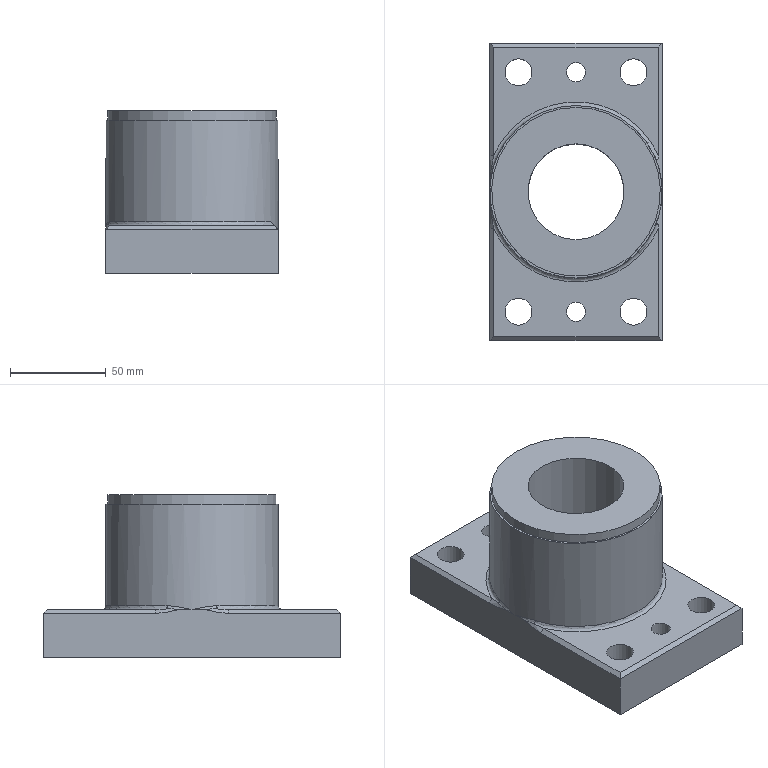Part | NX | features solid 2 | 1 solid | 30 faces | box 90 x 155 x 85 mm | volume 542156 mm3 | plane 15 | cylinder 9 | spline 4 | torus 2 | commonest cylinder face diameters 14 x4 10 x2 50 x1 88 x1 90 x1
STEP:
#1=CARTESIAN_POINT('',(325.,-795.,380.));
#2=VERTEX_POINT('',#1);
#3=CARTESIAN_POINT('',(325.,-770.,380.));
#4=DIRECTION('',(0.,0.,1.));
#5=DIRECTION('',(0.,-1.,0.));
#6=AXIS2_PLACEMENT_3D('',#3,#4,#5);
#7=CIRCLE('',#6,25.);
#8=EDGE_CURVE('',#2,#2,#7,.T.);
#9=ORIENTED_EDGE('',*,*,#8,.F.);
#10=EDGE_LOOP('',(#9));
#11=FACE_BOUND('',#10,.T.);
#12=CARTESIAN_POINT('',(325.,-726.,380.));
#13=VERTEX_POINT('',#12);
#14=CARTESIAN_POINT('',(325.,-770.,380.));
#15=DIRECTION('',(0.,0.,1.));
#16=DIRECTION('',(0.,1.,0.));
#17=AXIS2_PLACEMENT_3D('',#14,#15,#16);
#18=CIRCLE('',#17,44.);
#19=EDGE_CURVE('',#13,#13,#18,.T.);
#20=ORIENTED_EDGE('',*,*,#19,.T.);
#21=EDGE_LOOP('',(#20));
#22=FACE_BOUND('',#21,.T.);
#23=CARTESIAN_POINT('',(325.,-770.,380.));
#24=DIRECTION('',(0.,0.,1.));
#25=DIRECTION('',(0.,1.,0.));
#26=AXIS2_PLACEMENT_3D('',#23,#24,#25);
#27=PLANE('',#26);
#28=ADVANCED_FACE('',(#11,#22),#27,.T.);
#29=ORIENTED_EDGE('',*,*,#8,.T.);
#30=EDGE_LOOP('',(#29));
#31=FACE_BOUND('',#30,.T.);
#32=CARTESIAN_POINT('',(325.,-795.,295.));
#33=VERTEX_POINT('',#32);
#34=CARTESIAN_POINT('',(325.,-770.,295.));
#35=DIRECTION('',(0.,0.,1.));
#36=DIRECTION('',(0.,-1.,0.));
#37=AXIS2_PLACEMENT_3D('',#34,#35,#36);
#38=CIRCLE('',#37,25.);
#39=EDGE_CURVE('',#33,#33,#38,.T.);
#40=ORIENTED_EDGE('',*,*,#39,.F.);
#41=EDGE_LOOP('',(#40));
#42=FACE_BOUND('',#41,.T.);
#43=CARTESIAN_POINT('',(325.,-770.,380.));
#44=DIRECTION('',(0.,0.,-1.));
#45=DIRECTION('',(0.,-1.,0.));
#46=AXIS2_PLACEMENT_3D('',#43,#44,#45);
#47=CYLINDRICAL_SURFACE('',#46,25.);
#48=ADVANCED_FACE('',(#31,#42),#47,.F.);
#49=CARTESIAN_POINT('',(325.,-815.,375.));
#50=VERTEX_POINT('',#49);
#51=CARTESIAN_POINT('',(325.,-770.,375.));
#52=DIRECTION('',(0.,0.,1.));
#53=DIRECTION('',(0.,-1.,0.));
#54=AXIS2_PLACEMENT_3D('',#51,#52,#53);
#55=CIRCLE('',#54,45.);
#56=EDGE_CURVE('',#50,#50,#55,.T.);
#57=ORIENTED_EDGE('',*,*,#56,.F.);
#58=EDGE_LOOP('',(#57));
#59=FACE_BOUND('',#58,.T.);
#60=CARTESIAN_POINT('',(281.915,-757.013,322.));
#61=VERTEX_POINT('',#60);
#62=CARTESIAN_POINT('',(280.,-770.,320.));
#63=VERTEX_POINT('',#62);
#64=CARTESIAN_POINT('',(281.915,-757.013,322.));
#65=CARTESIAN_POINT('',(281.266,-759.164,322.));
#66=CARTESIAN_POINT('',(280.319,-763.441,321.407));
#67=CARTESIAN_POINT('',(280.,-767.835,320.466));
#68=CARTESIAN_POINT('',(280.,-770.,320.));
#69=B_SPLINE_CURVE_WITH_KNOTS('',3,(#64,#65,#66,#67,#68),.UNSPECIFIED.,.F.,.F.,(4,1,4),(0.,0.006644,0.01329),.UNSPECIFIED.);
#70=EDGE_CURVE('',#61,#63,#69,.T.);
#71=ORIENTED_EDGE('',*,*,#70,.T.);
#72=CARTESIAN_POINT('',(281.915,-782.987,322.));
#73=VERTEX_POINT('',#72);
#74=CARTESIAN_POINT('',(281.915,-782.987,322.));
#75=CARTESIAN_POINT('',(281.266,-780.836,322.));
#76=CARTESIAN_POINT('',(280.319,-776.559,321.407));
#77=CARTESIAN_POINT('',(280.,-772.165,320.466));
#78=CARTESIAN_POINT('',(280.,-770.,320.));
#79=B_SPLINE_CURVE_WITH_KNOTS('',3,(#74,#75,#76,#77,#78),.UNSPECIFIED.,.F.,.F.,(4,1,4),(0.,0.006644,0.01329),.UNSPECIFIED.);
#80=EDGE_CURVE('',#63,#73,#79,.F.);
#81=ORIENTED_EDGE('',*,*,#80,.T.);
#82=CARTESIAN_POINT('',(366.,-788.547,322.));
#83=VERTEX_POINT('',#82);
#84=CARTESIAN_POINT('',(325.,-770.,322.));
#85=DIRECTION('',(0.,0.,1.));
#86=DIRECTION('',(0.,1.,0.));
#87=AXIS2_PLACEMENT_3D('',#84,#85,#86);
#88=CIRCLE('',#87,45.);
#89=EDGE_CURVE('',#73,#83,#88,.T.);
#90=ORIENTED_EDGE('',*,*,#89,.T.);
#91=CARTESIAN_POINT('',(366.,-751.453,322.));
#92=VERTEX_POINT('',#91);
#93=CARTESIAN_POINT('',(325.,-770.,363.));
#94=DIRECTION('',(0.7071,0.,0.7071));
#95=DIRECTION('',(0.7071,0.,-0.7071));
#96=AXIS2_PLACEMENT_3D('',#93,#94,#95);
#97=ELLIPSE('',#96,63.64,45.);
#98=EDGE_CURVE('',#83,#92,#97,.T.);
#99=ORIENTED_EDGE('',*,*,#98,.T.);
#100=CARTESIAN_POINT('',(325.,-770.,322.));
#101=DIRECTION('',(0.,0.,1.));
#102=DIRECTION('',(0.,1.,0.));
#103=AXIS2_PLACEMENT_3D('',#100,#101,#102);
#104=CIRCLE('',#103,45.);
#105=EDGE_CURVE('',#92,#61,#104,.T.);
#106=ORIENTED_EDGE('',*,*,#105,.T.);
#107=EDGE_LOOP('',(#71,#81,#90,#99,#106));
#108=FACE_BOUND('',#107,.T.);
#109=CARTESIAN_POINT('',(325.,-770.,380.));
#110=DIRECTION('',(0.,0.,-1.));
#111=DIRECTION('',(0.,-1.,0.));
#112=AXIS2_PLACEMENT_3D('',#109,#110,#111);
#113=CYLINDRICAL_SURFACE('',#112,45.);
#114=ADVANCED_FACE('',(#59,#108),#113,.T.);
#115=CARTESIAN_POINT('',(355.,-700.5,320.));
#116=VERTEX_POINT('',#115);
#117=CARTESIAN_POINT('',(355.,-707.5,320.));
#118=DIRECTION('',(0.,0.,-1.));
#119=DIRECTION('',(0.,1.,0.));
#120=AXIS2_PLACEMENT_3D('',#117,#118,#119);
#121=CIRCLE('',#120,7.);
#122=EDGE_CURVE('',#116,#116,#121,.T.);
#123=ORIENTED_EDGE('',*,*,#122,.T.);
#124=EDGE_LOOP('',(#123));
#125=FACE_BOUND('',#124,.T.);
#126=CARTESIAN_POINT('',(325.,-702.5,320.));
#127=VERTEX_POINT('',#126);
#128=CARTESIAN_POINT('',(325.,-707.5,320.));
#129=DIRECTION('',(0.,0.,-1.));
#130=DIRECTION('',(0.,1.,0.));
#131=AXIS2_PLACEMENT_3D('',#128,#129,#130);
#132=CIRCLE('',#131,5.);
#133=EDGE_CURVE('',#127,#127,#132,.T.);
#134=ORIENTED_EDGE('',*,*,#133,.T.);
#135=EDGE_LOOP('',(#134));
#136=FACE_BOUND('',#135,.T.);
#137=CARTESIAN_POINT('',(295.,-700.5,320.));
#138=VERTEX_POINT('',#137);
#139=CARTESIAN_POINT('',(295.,-707.5,320.));
#140=DIRECTION('',(0.,0.,1.));
#141=DIRECTION('',(0.,1.,0.));
#142=AXIS2_PLACEMENT_3D('',#139,#140,#141);
#143=CIRCLE('',#142,7.);
#144=EDGE_CURVE('',#138,#138,#143,.T.);
#145=ORIENTED_EDGE('',*,*,#144,.F.);
#146=EDGE_LOOP('',(#145));
#147=FACE_BOUND('',#146,.T.);
#148=CARTESIAN_POINT('',(368.,-694.5,320.));
#149=VERTEX_POINT('',#148);
#150=CARTESIAN_POINT('',(282.,-694.5,320.));
#151=VERTEX_POINT('',#150);
#152=CARTESIAN_POINT('',(280.,-694.5,320.));
#153=DIRECTION('',(-1.,0.,0.));
#154=VECTOR('',#153,1000.);
#155=LINE('',#152,#154);
#156=EDGE_CURVE('',#149,#151,#155,.T.);
#157=ORIENTED_EDGE('',*,*,#156,.T.);
#158=CARTESIAN_POINT('',(282.,-751.026,320.001));
#159=VERTEX_POINT('',#158);
#160=CARTESIAN_POINT('',(282.,-692.5,320.));
#161=DIRECTION('',(0.,-1.,0.));
#162=VECTOR('',#161,1000.);
#163=LINE('',#160,#162);
#164=EDGE_CURVE('',#151,#159,#163,.T.);
#165=ORIENTED_EDGE('',*,*,#164,.T.);
#166=CARTESIAN_POINT('',(368.,-751.026,320.));
#167=VERTEX_POINT('',#166);
#168=CARTESIAN_POINT('',(325.,-770.,320.));
#169=DIRECTION('',(0.,0.,1.));
#170=DIRECTION('',(0.,1.,0.));
#171=AXIS2_PLACEMENT_3D('',#168,#169,#170);
#172=CIRCLE('',#171,47.);
#173=EDGE_CURVE('',#159,#167,#172,.F.);
#174=ORIENTED_EDGE('',*,*,#173,.T.);
#175=CARTESIAN_POINT('',(368.,-692.5,320.));
#176=DIRECTION('',(0.,1.,0.));
#177=VECTOR('',#176,1000.);
#178=LINE('',#175,#177);
#179=EDGE_CURVE('',#167,#149,#178,.T.);
#180=ORIENTED_EDGE('',*,*,#179,.T.);
#181=EDGE_LOOP('',(#157,#165,#174,#180));
#182=FACE_BOUND('',#181,.T.);
#183=CARTESIAN_POINT('',(370.,-692.5,320.));
#184=DIRECTION('',(0.,0.,1.));
#185=DIRECTION('',(0.,1.,0.));
#186=AXIS2_PLACEMENT_3D('',#183,#184,#185);
#187=PLANE('',#186);
#188=ADVANCED_FACE('',(#125,#136,#147,#182),#187,.T.);
#189=CARTESIAN_POINT('',(295.,-839.5,320.));
#190=VERTEX_POINT('',#189);
#191=CARTESIAN_POINT('',(295.,-832.5,320.));
#192=DIRECTION('',(0.,0.,-1.));
#193=DIRECTION('',(0.,-1.,0.));
#194=AXIS2_PLACEMENT_3D('',#191,#192,#193);
#195=CIRCLE('',#194,7.);
#196=EDGE_CURVE('',#190,#190,#195,.T.);
#197=ORIENTED_EDGE('',*,*,#196,.T.);
#198=EDGE_LOOP('',(#197));
#199=FACE_BOUND('',#198,.T.);
#200=CARTESIAN_POINT('',(355.,-839.5,320.));
#201=VERTEX_POINT('',#200);
#202=CARTESIAN_POINT('',(355.,-832.5,320.));
#203=DIRECTION('',(0.,0.,1.));
#204=DIRECTION('',(0.,-1.,0.));
#205=AXIS2_PLACEMENT_3D('',#202,#203,#204);
#206=CIRCLE('',#205,7.);
#207=EDGE_CURVE('',#201,#201,#206,.T.);
#208=ORIENTED_EDGE('',*,*,#207,.F.);
#209=EDGE_LOOP('',(#208));
#210=FACE_BOUND('',#209,.T.);
#211=CARTESIAN_POINT('',(325.,-837.5,320.));
#212=VERTEX_POINT('',#211);
#213=CARTESIAN_POINT('',(325.,-832.5,320.));
#214=DIRECTION('',(0.,0.,1.));
#215=DIRECTION('',(0.,-1.,0.));
#216=AXIS2_PLACEMENT_3D('',#213,#214,#215);
#217=CIRCLE('',#216,5.);
#218=EDGE_CURVE('',#212,#212,#217,.T.);
#219=ORIENTED_EDGE('',*,*,#218,.F.);
#220=EDGE_LOOP('',(#219));
#221=FACE_BOUND('',#220,.T.);
#222=CARTESIAN_POINT('',(368.,-788.974,320.));
#223=VERTEX_POINT('',#222);
#224=CARTESIAN_POINT('',(282.,-788.974,320.));
#225=VERTEX_POINT('',#224);
#226=CARTESIAN_POINT('',(325.,-770.,320.));
#227=DIRECTION('',(0.,0.,1.));
#228=DIRECTION('',(0.,1.,0.));
#229=AXIS2_PLACEMENT_3D('',#226,#227,#228);
#230=CIRCLE('',#229,47.);
#231=EDGE_CURVE('',#223,#225,#230,.F.);
#232=ORIENTED_EDGE('',*,*,#231,.T.);
#233=CARTESIAN_POINT('',(282.,-845.5,320.));
#234=VERTEX_POINT('',#233);
#235=CARTESIAN_POINT('',(282.,-692.5,320.));
#236=DIRECTION('',(0.,-1.,0.));
#237=VECTOR('',#236,1000.);
#238=LINE('',#235,#237);
#239=EDGE_CURVE('',#225,#234,#238,.T.);
#240=ORIENTED_EDGE('',*,*,#239,.T.);
#241=CARTESIAN_POINT('',(368.,-845.5,320.));
#242=VERTEX_POINT('',#241);
#243=CARTESIAN_POINT('',(368.,-845.5,320.));
#244=DIRECTION('',(1.,0.,0.));
#245=VECTOR('',#244,1000.);
#246=LINE('',#243,#245);
#247=EDGE_CURVE('',#234,#242,#246,.T.);
#248=ORIENTED_EDGE('',*,*,#247,.T.);
#249=CARTESIAN_POINT('',(368.,-692.5,320.));
#250=DIRECTION('',(0.,1.,0.));
#251=VECTOR('',#250,1000.);
#252=LINE('',#249,#251);
#253=EDGE_CURVE('',#242,#223,#252,.T.);
#254=ORIENTED_EDGE('',*,*,#253,.T.);
#255=EDGE_LOOP('',(#232,#240,#248,#254));
#256=FACE_BOUND('',#255,.T.);
#257=CARTESIAN_POINT('',(370.,-692.5,320.));
#258=DIRECTION('',(0.,0.,1.));
#259=DIRECTION('',(0.,1.,0.));
#260=AXIS2_PLACEMENT_3D('',#257,#258,#259);
#261=PLANE('',#260);
#262=ADVANCED_FACE('',(#199,#210,#221,#256),#261,.T.);
#263=CARTESIAN_POINT('',(370.,-847.5,318.));
#264=VERTEX_POINT('',#263);
#265=CARTESIAN_POINT('',(370.,-847.5,295.));
#266=VERTEX_POINT('',#265);
#267=CARTESIAN_POINT('',(370.,-847.5,320.));
#268=DIRECTION('',(0.,0.,-1.));
#269=VECTOR('',#268,1000.);
#270=LINE('',#267,#269);
#271=EDGE_CURVE('',#264,#266,#270,.T.);
#272=ORIENTED_EDGE('',*,*,#271,.F.);
#273=CARTESIAN_POINT('',(280.,-847.5,318.));
#274=VERTEX_POINT('',#273);
#275=CARTESIAN_POINT('',(280.,-847.5,318.));
#276=DIRECTION('',(-1.,0.,0.));
#277=VECTOR('',#276,1000.);
#278=LINE('',#275,#277);
#279=EDGE_CURVE('',#264,#274,#278,.T.);
#280=ORIENTED_EDGE('',*,*,#279,.T.);
#281=CARTESIAN_POINT('',(280.,-847.5,295.));
#282=VERTEX_POINT('',#281);
#283=CARTESIAN_POINT('',(280.,-847.5,320.));
#284=DIRECTION('',(0.,0.,-1.));
#285=VECTOR('',#284,1000.);
#286=LINE('',#283,#285);
#287=EDGE_CURVE('',#274,#282,#286,.T.);
#288=ORIENTED_EDGE('',*,*,#287,.T.);
#289=CARTESIAN_POINT('',(280.,-847.5,295.));
#290=DIRECTION('',(1.,0.,0.));
#291=VECTOR('',#290,1000.);
#292=LINE('',#289,#291);
#293=EDGE_CURVE('',#282,#266,#292,.T.);
#294=ORIENTED_EDGE('',*,*,#293,.T.);
#295=EDGE_LOOP('',(#272,#280,#288,#294));
#296=FACE_BOUND('',#295,.T.);
#297=CARTESIAN_POINT('',(280.,-847.5,320.));
#298=DIRECTION('',(0.,1.,0.));
#299=DIRECTION('',(1.,0.,0.));
#300=AXIS2_PLACEMENT_3D('',#297,#298,#299);
#301=PLANE('',#300);
#302=ADVANCED_FACE('',(#296),#301,.F.);
#303=ORIENTED_EDGE('',*,*,#287,.F.);
#304=CARTESIAN_POINT('',(280.,-788.974,318.002));
#305=VERTEX_POINT('',#304);
#306=CARTESIAN_POINT('',(280.,-770.,318.));
#307=DIRECTION('',(0.,1.,0.));
#308=VECTOR('',#307,1000.);
#309=LINE('',#306,#308);
#310=EDGE_CURVE('',#274,#305,#309,.T.);
#311=ORIENTED_EDGE('',*,*,#310,.T.);
#312=CARTESIAN_POINT('',(280.,-776.81,320.));
#313=VERTEX_POINT('',#312);
#314=CARTESIAN_POINT('',(280.,-788.974,318.003));
#315=CARTESIAN_POINT('',(280.,-788.028,318.007));
#316=CARTESIAN_POINT('',(280.,-786.557,318.084));
#317=CARTESIAN_POINT('',(280.,-784.716,318.306));
#318=CARTESIAN_POINT('',(280.,-783.668,318.463));
#319=CARTESIAN_POINT('',(280.,-782.774,318.617));
#320=CARTESIAN_POINT('',(280.,-782.221,318.722));
#321=CARTESIAN_POINT('',(280.,-781.307,318.906));
#322=CARTESIAN_POINT('',(280.,-779.648,319.272));
#323=CARTESIAN_POINT('',(280.,-777.997,319.684));
#324=CARTESIAN_POINT('',(280.,-776.81,320.));
#325=B_SPLINE_CURVE_WITH_KNOTS('',3,(#314,#315,#316,#317,#318,#319,#320,#321,#322,#323,#324),.UNSPECIFIED.,.F.,.F.,(4,1,1,1,1,1,1,1,4),(0.,0.25,0.375,0.4375,0.5,0.5625,0.625,0.75,1.),.UNSPECIFIED.);
#326=EDGE_CURVE('',#305,#313,#325,.T.);
#327=ORIENTED_EDGE('',*,*,#326,.T.);
#328=CARTESIAN_POINT('',(280.,-770.,320.));
#329=DIRECTION('',(0.,1.,0.));
#330=VECTOR('',#329,1000.);
#331=LINE('',#328,#330);
#332=EDGE_CURVE('',#313,#63,#331,.T.);
#333=ORIENTED_EDGE('',*,*,#332,.T.);
#334=CARTESIAN_POINT('',(280.,-763.19,320.));
#335=VERTEX_POINT('',#334);
#336=CARTESIAN_POINT('',(280.,-770.,320.));
#337=DIRECTION('',(0.,1.,0.));
#338=VECTOR('',#337,1000.);
#339=LINE('',#336,#338);
#340=EDGE_CURVE('',#63,#335,#339,.T.);
#341=ORIENTED_EDGE('',*,*,#340,.T.);
#342=CARTESIAN_POINT('',(280.,-751.026,318.003));
#343=VERTEX_POINT('',#342);
#344=CARTESIAN_POINT('',(280.,-763.19,320.));
#345=CARTESIAN_POINT('',(280.,-762.009,319.685));
#346=CARTESIAN_POINT('',(280.,-760.362,319.274));
#347=CARTESIAN_POINT('',(280.,-758.699,318.907));
#348=CARTESIAN_POINT('',(280.,-757.781,318.723));
#349=CARTESIAN_POINT('',(280.,-757.222,318.617));
#350=CARTESIAN_POINT('',(280.,-756.328,318.463));
#351=CARTESIAN_POINT('',(280.,-755.278,318.305));
#352=CARTESIAN_POINT('',(280.,-753.437,318.083));
#353=CARTESIAN_POINT('',(280.,-751.969,318.006));
#354=CARTESIAN_POINT('',(280.,-751.026,318.003));
#355=B_SPLINE_CURVE_WITH_KNOTS('',3,(#344,#345,#346,#347,#348,#349,#350,#351,#352,#353,#354),.UNSPECIFIED.,.F.,.F.,(4,1,1,1,1,1,1,1,4),(0.,0.25,0.375,0.4375,0.5,0.5625,0.625,0.75,1.),.UNSPECIFIED.);
#356=EDGE_CURVE('',#335,#343,#355,.T.);
#357=ORIENTED_EDGE('',*,*,#356,.T.);
#358=CARTESIAN_POINT('',(280.,-692.5,318.));
#359=VERTEX_POINT('',#358);
#360=CARTESIAN_POINT('',(280.,-770.,318.));
#361=DIRECTION('',(0.,1.,0.));
#362=VECTOR('',#361,1000.);
#363=LINE('',#360,#362);
#364=EDGE_CURVE('',#343,#359,#363,.T.);
#365=ORIENTED_EDGE('',*,*,#364,.T.);
#366=CARTESIAN_POINT('',(280.,-692.5,295.));
#367=VERTEX_POINT('',#366);
#368=CARTESIAN_POINT('',(280.,-692.5,320.));
#369=DIRECTION('',(0.,0.,-1.));
#370=VECTOR('',#369,1000.);
#371=LINE('',#368,#370);
#372=EDGE_CURVE('',#359,#367,#371,.T.);
#373=ORIENTED_EDGE('',*,*,#372,.T.);
#374=CARTESIAN_POINT('',(280.,-770.,295.));
#375=DIRECTION('',(0.,1.,0.));
#376=VECTOR('',#375,1000.);
#377=LINE('',#374,#376);
#378=EDGE_CURVE('',#282,#367,#377,.T.);
#379=ORIENTED_EDGE('',*,*,#378,.F.);
#380=EDGE_LOOP('',(#303,#311,#327,#333,#341,#357,#365,#373,#379));
#381=FACE_BOUND('',#380,.T.);
#382=CARTESIAN_POINT('',(280.,-770.,320.));
#383=DIRECTION('',(-1.,0.,0.));
#384=DIRECTION('',(0.,1.,0.));
#385=AXIS2_PLACEMENT_3D('',#382,#383,#384);
#386=PLANE('',#385);
#387=ADVANCED_FACE('',(#381),#386,.T.);
#388=ORIENTED_EDGE('',*,*,#372,.F.);
#389=CARTESIAN_POINT('',(370.,-692.5,318.));
#390=VERTEX_POINT('',#389);
#391=CARTESIAN_POINT('',(368.,-692.5,318.));
#392=DIRECTION('',(1.,0.,0.));
#393=VECTOR('',#392,1000.);
#394=LINE('',#391,#393);
#395=EDGE_CURVE('',#359,#390,#394,.T.);
#396=ORIENTED_EDGE('',*,*,#395,.T.);
#397=CARTESIAN_POINT('',(370.,-692.5,295.));
#398=VERTEX_POINT('',#397);
#399=CARTESIAN_POINT('',(370.,-692.5,320.));
#400=DIRECTION('',(0.,0.,-1.));
#401=VECTOR('',#400,1000.);
#402=LINE('',#399,#401);
#403=EDGE_CURVE('',#390,#398,#402,.T.);
#404=ORIENTED_EDGE('',*,*,#403,.T.);
#405=CARTESIAN_POINT('',(370.,-692.5,295.));
#406=DIRECTION('',(-1.,0.,0.));
#407=VECTOR('',#406,1000.);
#408=LINE('',#405,#407);
#409=EDGE_CURVE('',#398,#367,#408,.T.);
#410=ORIENTED_EDGE('',*,*,#409,.T.);
#411=EDGE_LOOP('',(#388,#396,#404,#410));
#412=FACE_BOUND('',#411,.T.);
#413=CARTESIAN_POINT('',(370.,-692.5,320.));
#414=DIRECTION('',(0.,-1.,0.));
#415=DIRECTION('',(-1.,0.,0.));
#416=AXIS2_PLACEMENT_3D('',#413,#414,#415);
#417=PLANE('',#416);
#418=ADVANCED_FACE('',(#412),#417,.F.);
#419=ORIENTED_EDGE('',*,*,#196,.F.);
#420=EDGE_LOOP('',(#419));
#421=FACE_BOUND('',#420,.T.);
#422=CARTESIAN_POINT('',(295.,-839.5,295.));
#423=VERTEX_POINT('',#422);
#424=CARTESIAN_POINT('',(295.,-832.5,295.));
#425=DIRECTION('',(0.,0.,-1.));
#426=DIRECTION('',(0.,-1.,0.));
#427=AXIS2_PLACEMENT_3D('',#424,#425,#426);
#428=CIRCLE('',#427,7.);
#429=EDGE_CURVE('',#423,#423,#428,.T.);
#430=ORIENTED_EDGE('',*,*,#429,.T.);
#431=EDGE_LOOP('',(#430));
#432=FACE_BOUND('',#431,.T.);
#433=CARTESIAN_POINT('',(295.,-832.5,320.));
#434=DIRECTION('',(0.,0.,-1.));
#435=DIRECTION('',(0.,-1.,0.));
#436=AXIS2_PLACEMENT_3D('',#433,#434,#435);
#437=CYLINDRICAL_SURFACE('',#436,7.);
#438=ADVANCED_FACE('',(#421,#432),#437,.F.);
#439=ORIENTED_EDGE('',*,*,#207,.T.);
#440=EDGE_LOOP('',(#439));
#441=FACE_BOUND('',#440,.T.);
#442=CARTESIAN_POINT('',(355.,-839.5,295.));
#443=VERTEX_POINT('',#442);
#444=CARTESIAN_POINT('',(355.,-832.5,295.));
#445=DIRECTION('',(0.,0.,1.));
#446=DIRECTION('',(0.,-1.,0.));
#447=AXIS2_PLACEMENT_3D('',#444,#445,#446);
#448=CIRCLE('',#447,7.);
#449=EDGE_CURVE('',#443,#443,#448,.T.);
#450=ORIENTED_EDGE('',*,*,#449,.F.);
#451=EDGE_LOOP('',(#450));
#452=FACE_BOUND('',#451,.T.);
#453=CARTESIAN_POINT('',(355.,-832.5,320.));
#454=DIRECTION('',(0.,0.,-1.));
#455=DIRECTION('',(0.,-1.,0.));
#456=AXIS2_PLACEMENT_3D('',#453,#454,#455);
#457=CYLINDRICAL_SURFACE('',#456,7.);
#458=ADVANCED_FACE('',(#441,#452),#457,.F.);
#459=ORIENTED_EDGE('',*,*,#403,.F.);
#460=CARTESIAN_POINT('',(370.,-756.435,318.));
#461=DIRECTION('',(0.,-1.,0.));
#462=VECTOR('',#461,1000.);
#463=LINE('',#460,#462);
#464=EDGE_CURVE('',#390,#264,#463,.T.);
#465=ORIENTED_EDGE('',*,*,#464,.T.);
#466=ORIENTED_EDGE('',*,*,#271,.T.);
#467=CARTESIAN_POINT('',(370.,-770.,295.));
#468=DIRECTION('',(0.,1.,0.));
#469=VECTOR('',#468,1000.);
#470=LINE('',#467,#469);
#471=EDGE_CURVE('',#266,#398,#470,.T.);
#472=ORIENTED_EDGE('',*,*,#471,.T.);
#473=EDGE_LOOP('',(#459,#465,#466,#472));
#474=FACE_BOUND('',#473,.T.);
#475=CARTESIAN_POINT('',(370.,-770.,320.));
#476=DIRECTION('',(-1.,0.,0.));
#477=DIRECTION('',(0.,0.,-1.));
#478=AXIS2_PLACEMENT_3D('',#475,#476,#477);
#479=PLANE('',#478);
#480=ADVANCED_FACE('',(#474),#479,.F.);
#481=ORIENTED_EDGE('',*,*,#122,.F.);
#482=EDGE_LOOP('',(#481));
#483=FACE_BOUND('',#482,.T.);
#484=CARTESIAN_POINT('',(355.,-700.5,295.));
#485=VERTEX_POINT('',#484);
#486=CARTESIAN_POINT('',(355.,-707.5,295.));
#487=DIRECTION('',(0.,0.,-1.));
#488=DIRECTION('',(0.,1.,0.));
#489=AXIS2_PLACEMENT_3D('',#486,#487,#488);
#490=CIRCLE('',#489,7.);
#491=EDGE_CURVE('',#485,#485,#490,.T.);
#492=ORIENTED_EDGE('',*,*,#491,.T.);
#493=EDGE_LOOP('',(#492));
#494=FACE_BOUND('',#493,.T.);
#495=CARTESIAN_POINT('',(355.,-707.5,320.));
#496=DIRECTION('',(0.,0.,-1.));
#497=DIRECTION('',(0.,-1.,0.));
#498=AXIS2_PLACEMENT_3D('',#495,#496,#497);
#499=CYLINDRICAL_SURFACE('',#498,7.);
#500=ADVANCED_FACE('',(#483,#494),#499,.F.);
#501=ORIENTED_EDGE('',*,*,#133,.F.);
#502=EDGE_LOOP('',(#501));
#503=FACE_BOUND('',#502,.T.);
#504=CARTESIAN_POINT('',(325.,-702.5,295.));
#505=VERTEX_POINT('',#504);
#506=CARTESIAN_POINT('',(325.,-707.5,295.));
#507=DIRECTION('',(0.,0.,-1.));
#508=DIRECTION('',(0.,1.,0.));
#509=AXIS2_PLACEMENT_3D('',#506,#507,#508);
#510=CIRCLE('',#509,5.);
#511=EDGE_CURVE('',#505,#505,#510,.T.);
#512=ORIENTED_EDGE('',*,*,#511,.T.);
#513=EDGE_LOOP('',(#512));
#514=FACE_BOUND('',#513,.T.);
#515=CARTESIAN_POINT('',(325.,-707.5,320.));
#516=DIRECTION('',(0.,0.,-1.));
#517=DIRECTION('',(0.,-1.,0.));
#518=AXIS2_PLACEMENT_3D('',#515,#516,#517);
#519=CYLINDRICAL_SURFACE('',#518,5.);
#520=ADVANCED_FACE('',(#503,#514),#519,.F.);
#521=ORIENTED_EDGE('',*,*,#144,.T.);
#522=EDGE_LOOP('',(#521));
#523=FACE_BOUND('',#522,.T.);
#524=CARTESIAN_POINT('',(295.,-700.5,295.));
#525=VERTEX_POINT('',#524);
#526=CARTESIAN_POINT('',(295.,-707.5,295.));
#527=DIRECTION('',(0.,0.,1.));
#528=DIRECTION('',(0.,1.,0.));
#529=AXIS2_PLACEMENT_3D('',#526,#527,#528);
#530=CIRCLE('',#529,7.);
#531=EDGE_CURVE('',#525,#525,#530,.T.);
#532=ORIENTED_EDGE('',*,*,#531,.F.);
#533=EDGE_LOOP('',(#532));
#534=FACE_BOUND('',#533,.T.);
#535=CARTESIAN_POINT('',(295.,-707.5,320.));
#536=DIRECTION('',(0.,0.,-1.));
#537=DIRECTION('',(0.,-1.,0.));
#538=AXIS2_PLACEMENT_3D('',#535,#536,#537);
#539=CYLINDRICAL_SURFACE('',#538,7.);
#540=ADVANCED_FACE('',(#523,#534),#539,.F.);
#541=ORIENTED_EDGE('',*,*,#218,.T.);
#542=EDGE_LOOP('',(#541));
#543=FACE_BOUND('',#542,.T.);
#544=CARTESIAN_POINT('',(325.,-837.5,295.));
#545=VERTEX_POINT('',#544);
#546=CARTESIAN_POINT('',(325.,-832.5,295.));
#547=DIRECTION('',(0.,0.,1.));
#548=DIRECTION('',(0.,-1.,0.));
#549=AXIS2_PLACEMENT_3D('',#546,#547,#548);
#550=CIRCLE('',#549,5.);
#551=EDGE_CURVE('',#545,#545,#550,.T.);
#552=ORIENTED_EDGE('',*,*,#551,.F.);
#553=EDGE_LOOP('',(#552));
#554=FACE_BOUND('',#553,.T.);
#555=CARTESIAN_POINT('',(325.,-832.5,320.));
#556=DIRECTION('',(0.,0.,-1.));
#557=DIRECTION('',(0.,-1.,0.));
#558=AXIS2_PLACEMENT_3D('',#555,#556,#557);
#559=CYLINDRICAL_SURFACE('',#558,5.);
#560=ADVANCED_FACE('',(#543,#554),#559,.F.);
#561=ORIENTED_EDGE('',*,*,#551,.T.);
#562=EDGE_LOOP('',(#561));
#563=FACE_BOUND('',#562,.T.);
#564=ORIENTED_EDGE('',*,*,#531,.T.);
#565=EDGE_LOOP('',(#564));
#566=FACE_BOUND('',#565,.T.);
#567=ORIENTED_EDGE('',*,*,#511,.F.);
#568=EDGE_LOOP('',(#567));
#569=FACE_BOUND('',#568,.T.);
#570=ORIENTED_EDGE('',*,*,#491,.F.);
#571=EDGE_LOOP('',(#570));
#572=FACE_BOUND('',#571,.T.);
#573=ORIENTED_EDGE('',*,*,#471,.F.);
#574=ORIENTED_EDGE('',*,*,#293,.F.);
#575=ORIENTED_EDGE('',*,*,#378,.T.);
#576=ORIENTED_EDGE('',*,*,#409,.F.);
#577=EDGE_LOOP('',(#573,#574,#575,#576));
#578=FACE_BOUND('',#577,.T.);
#579=ORIENTED_EDGE('',*,*,#449,.T.);
#580=EDGE_LOOP('',(#579));
#581=FACE_BOUND('',#580,.T.);
#582=ORIENTED_EDGE('',*,*,#429,.F.);
#583=EDGE_LOOP('',(#582));
#584=FACE_BOUND('',#583,.T.);
#585=ORIENTED_EDGE('',*,*,#39,.T.);
#586=EDGE_LOOP('',(#585));
#587=FACE_BOUND('',#586,.T.);
#588=CARTESIAN_POINT('',(370.,-692.5,295.));
#589=DIRECTION('',(0.,0.,1.));
#590=DIRECTION('',(0.,1.,0.));
#591=AXIS2_PLACEMENT_3D('',#588,#589,#590);
#592=PLANE('',#591);
#593=ADVANCED_FACE('',(#563,#566,#569,#572,#578,#581,#584,#587),#592,.F.);
#594=CARTESIAN_POINT('',(280.999,-783.263,320.294));
#595=VERTEX_POINT('',#594);
#596=CARTESIAN_POINT('',(280.,-783.565,322.));
#597=DIRECTION('',(0.2886,-0.9574,0.));
#598=DIRECTION('',(-0.9574,-0.2886,0.));
#599=AXIS2_PLACEMENT_3D('',#596,#597,#598);
#600=CIRCLE('',#599,2.);
#601=EDGE_CURVE('',#595,#73,#600,.T.);
#602=ORIENTED_EDGE('',*,*,#601,.F.);
#603=CARTESIAN_POINT('',(280.999,-783.263,320.294));
#604=CARTESIAN_POINT('',(281.324,-785.466,320.095));
#605=CARTESIAN_POINT('',(281.678,-787.373,320.));
#606=CARTESIAN_POINT('',(282.,-788.974,320.));
#607=B_SPLINE_CURVE_WITH_KNOTS('',3,(#603,#604,#605,#606),.UNSPECIFIED.,.F.,.F.,(4,4),(0.,1.),.UNSPECIFIED.);
#608=EDGE_CURVE('',#595,#225,#607,.T.);
#609=ORIENTED_EDGE('',*,*,#608,.T.);
#610=ORIENTED_EDGE('',*,*,#231,.F.);
#611=CARTESIAN_POINT('',(368.,-788.974,320.));
#612=CARTESIAN_POINT('',(368.,-788.522,320.));
#613=CARTESIAN_POINT('',(367.96,-787.855,320.04));
#614=CARTESIAN_POINT('',(367.776,-786.963,320.224));
#615=CARTESIAN_POINT('',(367.318,-786.569,320.682));
#616=CARTESIAN_POINT('',(366.876,-786.987,321.124));
#617=CARTESIAN_POINT('',(366.447,-787.61,321.553));
#618=CARTESIAN_POINT('',(366.171,-788.17,321.829));
#619=CARTESIAN_POINT('',(366.,-788.547,322.));
#620=B_SPLINE_CURVE_WITH_KNOTS('',3,(#611,#612,#613,#614,#615,#616,#617,#618,#619),.UNSPECIFIED.,.F.,.F.,(4,1,1,1,1,1,4),(0.,0.00135,0.002025,0.0027,0.003375,0.00405,0.0054),.UNSPECIFIED.);
#621=EDGE_CURVE('',#223,#83,#620,.T.);
#622=ORIENTED_EDGE('',*,*,#621,.T.);
#623=ORIENTED_EDGE('',*,*,#89,.F.);
#624=EDGE_LOOP('',(#602,#609,#610,#622,#623));
#625=FACE_BOUND('',#624,.T.);
#626=CARTESIAN_POINT('',(325.,-770.,322.));
#627=DIRECTION('',(0.,0.,1.));
#628=DIRECTION('',(0.,1.,0.));
#629=AXIS2_PLACEMENT_3D('',#626,#627,#628);
#630=TOROIDAL_SURFACE('',#629,47.,2.);
#631=ADVANCED_FACE('',(#625),#630,.F.);
#632=ORIENTED_EDGE('',*,*,#332,.F.);
#633=CARTESIAN_POINT('',(281.,-783.263,320.293));
#634=CARTESIAN_POINT('',(280.648,-780.879,320.508));
#635=CARTESIAN_POINT('',(280.193,-778.668,320.22));
#636=CARTESIAN_POINT('',(280.,-776.81,320.));
#637=B_SPLINE_CURVE_WITH_KNOTS('',3,(#633,#634,#635,#636),.UNSPECIFIED.,.F.,.F.,(4,4),(0.,1.),.UNSPECIFIED.);
#638=EDGE_CURVE('',#313,#595,#637,.F.);
#639=ORIENTED_EDGE('',*,*,#638,.T.);
#640=ORIENTED_EDGE('',*,*,#601,.T.);
#641=ORIENTED_EDGE('',*,*,#80,.F.);
#642=EDGE_LOOP('',(#632,#639,#640,#641));
#643=FACE_BOUND('',#642,.T.);
#644=CARTESIAN_POINT('',(280.,-783.646,320.));
#645=CARTESIAN_POINT('',(281.936,-783.058,319.976));
#646=CARTESIAN_POINT('',(281.938,-783.065,322.));
#647=CARTESIAN_POINT('',(280.,-782.519,320.));
#648=CARTESIAN_POINT('',(281.661,-782.152,320.285));
#649=CARTESIAN_POINT('',(281.611,-781.986,322.004));
#650=CARTESIAN_POINT('',(280.,-780.269,320.));
#651=CARTESIAN_POINT('',(281.109,-780.116,320.608));
#652=CARTESIAN_POINT('',(281.045,-779.832,321.846));
#653=CARTESIAN_POINT('',(280.,-775.735,320.));
#654=CARTESIAN_POINT('',(280.285,-775.811,320.609));
#655=CARTESIAN_POINT('',(280.242,-775.491,321.187));
#656=CARTESIAN_POINT('',(280.,-772.332,320.));
#657=CARTESIAN_POINT('',(280.,-772.282,320.241));
#658=CARTESIAN_POINT('',(280.,-772.233,320.481));
#659=CARTESIAN_POINT('',(280.,-770.,320.));
#660=CARTESIAN_POINT('',(280.,-770.,320.));
#661=CARTESIAN_POINT('',(280.,-770.,320.));
#662=(BOUNDED_SURFACE()B_SPLINE_SURFACE(3,2,((#644,#645,#646),(#647,#648,#649),(#650,#651,#652),(#653,#654,#655),(#656,#657,#658),(#659,#660,#661)),.UNSPECIFIED.,.F.,.F.,.F.)B_SPLINE_SURFACE_WITH_KNOTS((4,1,1,4),(3,3),(0.006478,0.01005,0.01362,0.02076),(0.,1.),.UNSPECIFIED.)GEOMETRIC_REPRESENTATION_ITEM()RATIONAL_B_SPLINE_SURFACE(((1.,0.703,1.),(1.,0.7611,1.),(1.,0.8512,1.),(1.,0.9681,1.),(1.,1.,1.),(1.,1.,1.)))REPRESENTATION_ITEM('')SURFACE());
#663=ADVANCED_FACE('',(#643),#662,.F.);
#664=CARTESIAN_POINT('',(281.,-756.737,320.294));
#665=VERTEX_POINT('',#664);
#666=CARTESIAN_POINT('',(280.,-756.435,322.));
#667=DIRECTION('',(0.2886,0.9574,0.));
#668=DIRECTION('',(0.9574,-0.2886,0.));
#669=AXIS2_PLACEMENT_3D('',#666,#667,#668);
#670=CIRCLE('',#669,2.);
#671=EDGE_CURVE('',#665,#61,#670,.F.);
#672=ORIENTED_EDGE('',*,*,#671,.F.);
#673=CARTESIAN_POINT('',(280.,-763.19,320.));
#674=CARTESIAN_POINT('',(280.193,-761.334,320.22));
#675=CARTESIAN_POINT('',(280.648,-759.121,320.508));
#676=CARTESIAN_POINT('',(281.,-756.737,320.293));
#677=B_SPLINE_CURVE_WITH_KNOTS('',3,(#673,#674,#675,#676),.UNSPECIFIED.,.F.,.F.,(4,4),(0.,1.),.UNSPECIFIED.);
#678=EDGE_CURVE('',#665,#335,#677,.F.);
#679=ORIENTED_EDGE('',*,*,#678,.T.);
#680=ORIENTED_EDGE('',*,*,#340,.F.);
#681=ORIENTED_EDGE('',*,*,#70,.F.);
#682=EDGE_LOOP('',(#672,#679,#680,#681));
#683=FACE_BOUND('',#682,.T.);
#684=CARTESIAN_POINT('',(281.938,-756.935,322.));
#685=CARTESIAN_POINT('',(281.936,-756.942,319.976));
#686=CARTESIAN_POINT('',(280.,-756.354,320.));
#687=CARTESIAN_POINT('',(281.611,-758.014,322.004));
#688=CARTESIAN_POINT('',(281.661,-757.848,320.285));
#689=CARTESIAN_POINT('',(280.,-757.481,320.));
#690=CARTESIAN_POINT('',(281.045,-760.168,321.846));
#691=CARTESIAN_POINT('',(281.109,-759.884,320.608));
#692=CARTESIAN_POINT('',(280.,-759.731,320.));
#693=CARTESIAN_POINT('',(280.242,-764.509,321.187));
#694=CARTESIAN_POINT('',(280.285,-764.189,320.609));
#695=CARTESIAN_POINT('',(280.,-764.265,320.));
#696=CARTESIAN_POINT('',(280.,-767.767,320.481));
#697=CARTESIAN_POINT('',(280.,-767.718,320.241));
#698=CARTESIAN_POINT('',(280.,-767.668,320.));
#699=CARTESIAN_POINT('',(280.,-770.,320.));
#700=CARTESIAN_POINT('',(280.,-770.,320.));
#701=CARTESIAN_POINT('',(280.,-770.,320.));
#702=(BOUNDED_SURFACE()B_SPLINE_SURFACE(3,2,((#684,#685,#686),(#687,#688,#689),(#690,#691,#692),(#693,#694,#695),(#696,#697,#698),(#699,#700,#701)),.UNSPECIFIED.,.F.,.F.,.F.)B_SPLINE_SURFACE_WITH_KNOTS((4,1,1,4),(3,3),(0.006478,0.01005,0.01362,0.02076),(0.,1.),.UNSPECIFIED.)GEOMETRIC_REPRESENTATION_ITEM()RATIONAL_B_SPLINE_SURFACE(((1.,0.703,1.),(1.,0.7611,1.),(1.,0.8512,1.),(1.,0.9681,1.),(1.,1.,1.),(1.,1.,1.)))REPRESENTATION_ITEM('')SURFACE());
#703=ADVANCED_FACE('',(#683),#702,.F.);
#704=ORIENTED_EDGE('',*,*,#173,.F.);
#705=CARTESIAN_POINT('',(282.,-751.026,320.));
#706=CARTESIAN_POINT('',(281.676,-752.634,320.));
#707=CARTESIAN_POINT('',(281.323,-754.541,320.096));
#708=CARTESIAN_POINT('',(281.,-756.737,320.294));
#709=B_SPLINE_CURVE_WITH_KNOTS('',3,(#705,#706,#707,#708),.UNSPECIFIED.,.F.,.F.,(4,4),(0.,1.),.UNSPECIFIED.);
#710=EDGE_CURVE('',#159,#665,#709,.T.);
#711=ORIENTED_EDGE('',*,*,#710,.T.);
#712=ORIENTED_EDGE('',*,*,#671,.T.);
#713=ORIENTED_EDGE('',*,*,#105,.F.);
#714=CARTESIAN_POINT('',(366.,-751.453,322.));
#715=CARTESIAN_POINT('',(366.17,-751.829,321.83));
#716=CARTESIAN_POINT('',(366.443,-752.383,321.557));
#717=CARTESIAN_POINT('',(366.872,-753.007,321.128));
#718=CARTESIAN_POINT('',(367.313,-753.431,320.687));
#719=CARTESIAN_POINT('',(367.776,-753.04,320.224));
#720=CARTESIAN_POINT('',(367.961,-752.139,320.039));
#721=CARTESIAN_POINT('',(368.,-751.478,320.));
#722=CARTESIAN_POINT('',(368.,-751.026,320.));
#723=B_SPLINE_CURVE_WITH_KNOTS('',3,(#714,#715,#716,#717,#718,#719,#720,#721,#722),.UNSPECIFIED.,.F.,.F.,(4,1,1,1,1,1,4),(0.,0.001331,0.001996,0.002661,0.003327,0.003992,0.005323),.UNSPECIFIED.);
#724=EDGE_CURVE('',#92,#167,#723,.T.);
#725=ORIENTED_EDGE('',*,*,#724,.T.);
#726=EDGE_LOOP('',(#704,#711,#712,#713,#725));
#727=FACE_BOUND('',#726,.T.);
#728=CARTESIAN_POINT('',(325.,-770.,322.));
#729=DIRECTION('',(0.,0.,1.));
#730=DIRECTION('',(0.,1.,0.));
#731=AXIS2_PLACEMENT_3D('',#728,#729,#730);
#732=TOROIDAL_SURFACE('',#731,47.,2.);
#733=ADVANCED_FACE('',(#727),#732,.F.);
#734=ORIENTED_EDGE('',*,*,#464,.F.);
#735=CARTESIAN_POINT('',(368.667,-693.833,319.333));
#736=DIRECTION('',(-0.5774,-0.5774,0.5774));
#737=VECTOR('',#736,1000.);
#738=LINE('',#735,#737);
#739=EDGE_CURVE('',#390,#149,#738,.T.);
#740=ORIENTED_EDGE('',*,*,#739,.T.);
#741=ORIENTED_EDGE('',*,*,#179,.F.);
#742=ORIENTED_EDGE('',*,*,#724,.F.);
#743=ORIENTED_EDGE('',*,*,#98,.F.);
#744=ORIENTED_EDGE('',*,*,#621,.F.);
#745=ORIENTED_EDGE('',*,*,#253,.F.);
#746=CARTESIAN_POINT('',(317.,-794.5,371.));
#747=DIRECTION('',(0.5774,-0.5774,-0.5774));
#748=VECTOR('',#747,1000.);
#749=LINE('',#746,#748);
#750=EDGE_CURVE('',#242,#264,#749,.T.);
#751=ORIENTED_EDGE('',*,*,#750,.T.);
#752=EDGE_LOOP('',(#734,#740,#741,#742,#743,#744,#745,#751));
#753=FACE_BOUND('',#752,.T.);
#754=CARTESIAN_POINT('',(368.,-692.5,320.));
#755=DIRECTION('',(0.7071,0.,0.7071));
#756=DIRECTION('',(-0.7071,0.,0.7071));
#757=AXIS2_PLACEMENT_3D('',#754,#755,#756);
#758=PLANE('',#757);
#759=ADVANCED_FACE('',(#753),#758,.T.);
#760=ORIENTED_EDGE('',*,*,#395,.F.);
#761=CARTESIAN_POINT('',(311.333,-723.833,349.333));
#762=DIRECTION('',(-0.5774,0.5774,-0.5774));
#763=VECTOR('',#762,1000.);
#764=LINE('',#761,#763);
#765=EDGE_CURVE('',#359,#151,#764,.F.);
#766=ORIENTED_EDGE('',*,*,#765,.T.);
#767=ORIENTED_EDGE('',*,*,#156,.F.);
#768=ORIENTED_EDGE('',*,*,#739,.F.);
#769=EDGE_LOOP('',(#760,#766,#767,#768));
#770=FACE_BOUND('',#769,.T.);
#771=CARTESIAN_POINT('',(370.,-694.5,320.));
#772=DIRECTION('',(0.,0.7071,0.7071));
#773=DIRECTION('',(0.,0.7071,-0.7071));
#774=AXIS2_PLACEMENT_3D('',#771,#772,#773);
#775=PLANE('',#774);
#776=ADVANCED_FACE('',(#770),#775,.T.);
#777=ORIENTED_EDGE('',*,*,#247,.F.);
#778=CARTESIAN_POINT('',(311.333,-816.167,349.333));
#779=DIRECTION('',(0.5774,0.5774,0.5774));
#780=VECTOR('',#779,1000.);
#781=LINE('',#778,#780);
#782=EDGE_CURVE('',#234,#274,#781,.F.);
#783=ORIENTED_EDGE('',*,*,#782,.T.);
#784=ORIENTED_EDGE('',*,*,#279,.F.);
#785=ORIENTED_EDGE('',*,*,#750,.F.);
#786=EDGE_LOOP('',(#777,#783,#784,#785));
#787=FACE_BOUND('',#786,.T.);
#788=CARTESIAN_POINT('',(370.,-845.5,320.));
#789=DIRECTION('',(0.,-0.7071,0.7071));
#790=DIRECTION('',(0.,0.7071,0.7071));
#791=AXIS2_PLACEMENT_3D('',#788,#789,#790);
#792=PLANE('',#791);
#793=ADVANCED_FACE('',(#787),#792,.T.);
#794=ORIENTED_EDGE('',*,*,#765,.F.);
#795=ORIENTED_EDGE('',*,*,#364,.F.);
#796=CARTESIAN_POINT('',(280.002,-751.026,318.002));
#797=CARTESIAN_POINT('',(280.668,-751.026,318.668));
#798=CARTESIAN_POINT('',(281.334,-751.026,319.334));
#799=CARTESIAN_POINT('',(282.001,-751.026,320.001));
#800=B_SPLINE_CURVE_WITH_KNOTS('',3,(#796,#797,#798,#799),.UNSPECIFIED.,.F.,.F.,(4,4),(0.,1.),.UNSPECIFIED.);
#801=EDGE_CURVE('',#159,#343,#800,.F.);
#802=ORIENTED_EDGE('',*,*,#801,.F.);
#803=ORIENTED_EDGE('',*,*,#164,.F.);
#804=EDGE_LOOP('',(#794,#795,#802,#803));
#805=FACE_BOUND('',#804,.T.);
#806=CARTESIAN_POINT('',(280.,-770.,318.));
#807=DIRECTION('',(0.7071,0.,-0.7071));
#808=DIRECTION('',(0.7071,0.,0.7071));
#809=AXIS2_PLACEMENT_3D('',#806,#807,#808);
#810=PLANE('',#809);
#811=ADVANCED_FACE('',(#805),#810,.F.);
#812=ORIENTED_EDGE('',*,*,#678,.F.);
#813=ORIENTED_EDGE('',*,*,#710,.F.);
#814=ORIENTED_EDGE('',*,*,#801,.T.);
#815=ORIENTED_EDGE('',*,*,#356,.F.);
#816=EDGE_LOOP('',(#812,#813,#814,#815));
#817=FACE_BOUND('',#816,.T.);
#818=CARTESIAN_POINT('',(280.,-763.19,320.));
#819=CARTESIAN_POINT('',(280.,-759.186,318.933));
#820=CARTESIAN_POINT('',(280.,-755.112,318.005));
#821=CARTESIAN_POINT('',(280.,-750.952,318.003));
#822=CARTESIAN_POINT('',(280.289,-762.919,321.));
#823=CARTESIAN_POINT('',(280.621,-758.806,320.467));
#824=CARTESIAN_POINT('',(281.243,-754.773,320.003));
#825=CARTESIAN_POINT('',(282.014,-750.958,320.002));
#826=B_SPLINE_SURFACE_WITH_KNOTS('',1,3,((#818,#819,#820,#821),(#822,#823,#824,#825)),.RULED_SURF.,.F.,.F.,.F.,(2,2),(4,4),(0.,1.),(-0.0006167,0.01179),.PIECEWISE_BEZIER_KNOTS.);
#827=ADVANCED_FACE('',(#817),#826,.T.);
#828=ORIENTED_EDGE('',*,*,#638,.F.);
#829=ORIENTED_EDGE('',*,*,#326,.F.);
#830=CARTESIAN_POINT('',(282.,-788.974,320.));
#831=CARTESIAN_POINT('',(281.333,-788.974,319.333));
#832=CARTESIAN_POINT('',(280.667,-788.974,318.667));
#833=CARTESIAN_POINT('',(280.,-788.974,318.));
#834=B_SPLINE_CURVE_WITH_KNOTS('',3,(#830,#831,#832,#833),.UNSPECIFIED.,.F.,.F.,(4,4),(0.,1.),.UNSPECIFIED.);
#835=EDGE_CURVE('',#225,#305,#834,.T.);
#836=ORIENTED_EDGE('',*,*,#835,.F.);
#837=ORIENTED_EDGE('',*,*,#608,.F.);
#838=EDGE_LOOP('',(#828,#829,#836,#837));
#839=FACE_BOUND('',#838,.T.);
#840=CARTESIAN_POINT('',(279.986,-789.048,317.99));
#841=CARTESIAN_POINT('',(279.991,-784.867,317.994));
#842=CARTESIAN_POINT('',(279.996,-780.822,318.921));
#843=CARTESIAN_POINT('',(279.998,-776.808,319.993));
#844=CARTESIAN_POINT('',(280.,-789.048,318.003));
#845=CARTESIAN_POINT('',(280.,-784.869,318.007));
#846=CARTESIAN_POINT('',(280.,-780.825,318.932));
#847=CARTESIAN_POINT('',(280.,-776.81,320.));
#848=CARTESIAN_POINT('',(282.014,-789.043,320.002));
#849=CARTESIAN_POINT('',(281.24,-785.209,320.004));
#850=CARTESIAN_POINT('',(280.623,-781.205,320.466));
#851=CARTESIAN_POINT('',(280.289,-777.081,321.));
#852=B_SPLINE_SURFACE_WITH_KNOTS('',1,3,((#840,#841,#842,#843),(#844,#845,#846,#847),(#848,#849,#850,#851)),.RULED_SURF.,.F.,.F.,.F.,(2,1,2),(4,4),(-0.006878,0.,1.),(-0.01183,0.0006189),.PIECEWISE_BEZIER_KNOTS.);
#853=ADVANCED_FACE('',(#839),#852,.T.);
#854=ORIENTED_EDGE('',*,*,#782,.F.);
#855=ORIENTED_EDGE('',*,*,#239,.F.);
#856=ORIENTED_EDGE('',*,*,#835,.T.);
#857=ORIENTED_EDGE('',*,*,#310,.F.);
#858=EDGE_LOOP('',(#854,#855,#856,#857));
#859=FACE_BOUND('',#858,.T.);
#860=CARTESIAN_POINT('',(280.,-770.,318.));
#861=DIRECTION('',(0.7071,0.,-0.7071));
#862=DIRECTION('',(0.7071,0.,0.7071));
#863=AXIS2_PLACEMENT_3D('',#860,#861,#862);
#864=PLANE('',#863);
#865=ADVANCED_FACE('',(#859),#864,.F.);
#866=ORIENTED_EDGE('',*,*,#19,.F.);
#867=EDGE_LOOP('',(#866));
#868=FACE_BOUND('',#867,.T.);
#869=CARTESIAN_POINT('',(325.,-726.,375.));
#870=VERTEX_POINT('',#869);
#871=CARTESIAN_POINT('',(325.,-770.,375.));
#872=DIRECTION('',(0.,0.,1.));
#873=DIRECTION('',(0.,1.,0.));
#874=AXIS2_PLACEMENT_3D('',#871,#872,#873);
#875=CIRCLE('',#874,44.);
#876=EDGE_CURVE('',#870,#870,#875,.T.);
#877=ORIENTED_EDGE('',*,*,#876,.T.);
#878=EDGE_LOOP('',(#877));
#879=FACE_BOUND('',#878,.T.);
#880=CARTESIAN_POINT('',(325.,-770.,375.));
#881=DIRECTION('',(0.,0.,1.));
#882=DIRECTION('',(0.,1.,0.));
#883=AXIS2_PLACEMENT_3D('',#880,#881,#882);
#884=CYLINDRICAL_SURFACE('',#883,44.);
#885=ADVANCED_FACE('',(#868,#879),#884,.T.);
#886=ORIENTED_EDGE('',*,*,#876,.F.);
#887=EDGE_LOOP('',(#886));
#888=FACE_BOUND('',#887,.T.);
#889=ORIENTED_EDGE('',*,*,#56,.T.);
#890=EDGE_LOOP('',(#889));
#891=FACE_BOUND('',#890,.T.);
#892=CARTESIAN_POINT('',(325.,-770.,375.));
#893=DIRECTION('',(0.,0.,-1.));
#894=DIRECTION('',(0.,-1.,0.));
#895=AXIS2_PLACEMENT_3D('',#892,#893,#894);
#896=PLANE('',#895);
#897=ADVANCED_FACE('',(#888,#891),#896,.F.);
#898=CLOSED_SHELL('',(#28,#48,#114,#188,#262,#302,#387,#418,#438,#458,#480,#500,#520,#540,#560,#593,#631,#663,#703,#733,#759,#776,#793,#811,#827,#853,#865,#885,#897));
#899=MANIFOLD_SOLID_BREP('',#898);
#900=(LENGTH_UNIT()NAMED_UNIT(*)SI_UNIT(.MILLI.,.METRE.));
#901=UNCERTAINTY_MEASURE_WITH_UNIT(LENGTH_MEASURE(0.1051),#900,'','');
#902=(NAMED_UNIT(*)PLANE_ANGLE_UNIT()SI_UNIT($,.RADIAN.));
#903=(NAMED_UNIT(*)SI_UNIT($,.STERADIAN.)SOLID_ANGLE_UNIT());
#904=(GEOMETRIC_REPRESENTATION_CONTEXT(3)GLOBAL_UNCERTAINTY_ASSIGNED_CONTEXT((#901))GLOBAL_UNIT_ASSIGNED_CONTEXT((#900,#902,#903))REPRESENTATION_CONTEXT('',''));
#905=ADVANCED_BREP_SHAPE_REPRESENTATION('',(#899),#904);